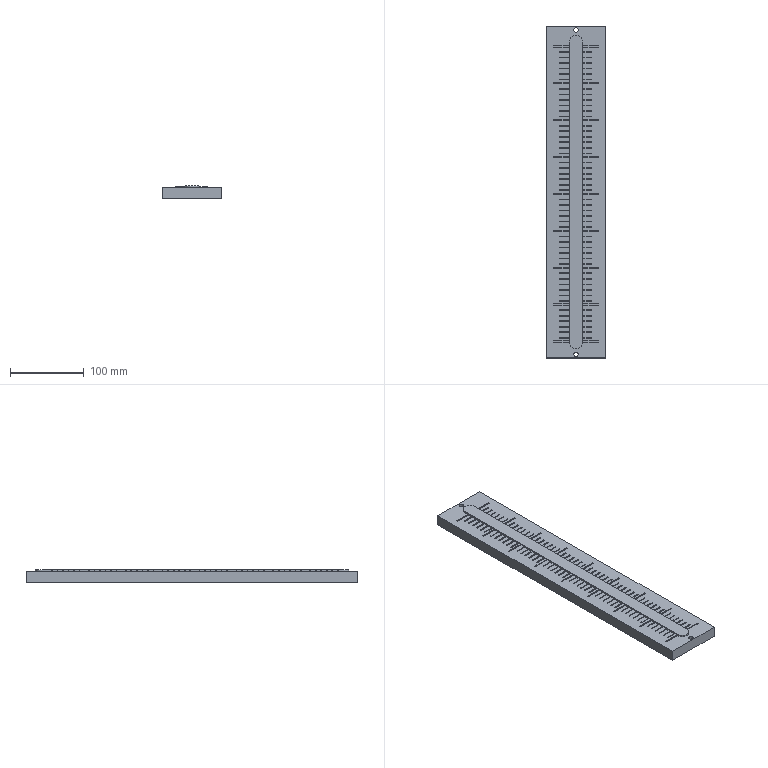Part | SolidWorks | features ICE 3, Extrusion 1, LPattern 1 | 1 solid | 471 faces | box 80 x 450 x 17 mm | volume 554690 mm3 | plane 465 | cylinder 6 | commonest cylinder face diameters 6 x4 18.197 x2